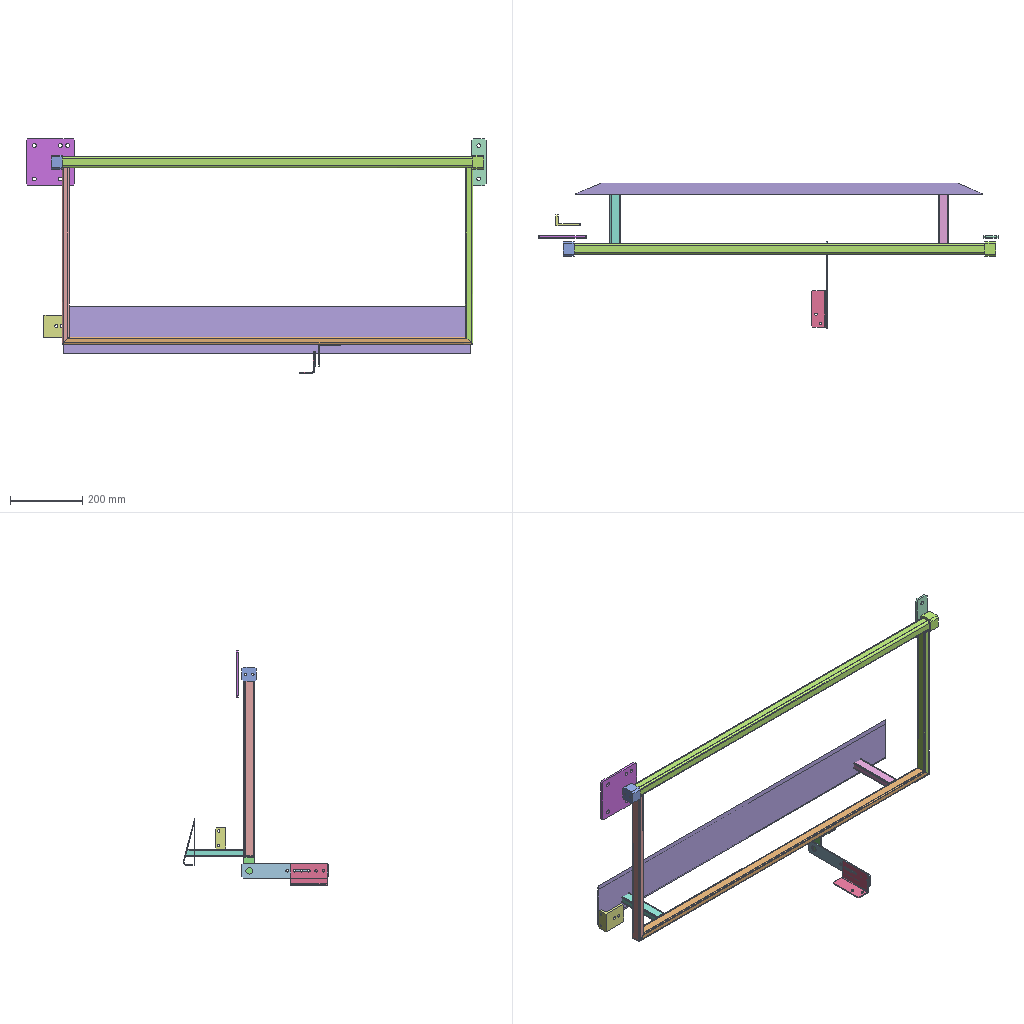Assembly | SolidWorks | 8 different items | 8 placed | box 1271 x 403 x 648 mm
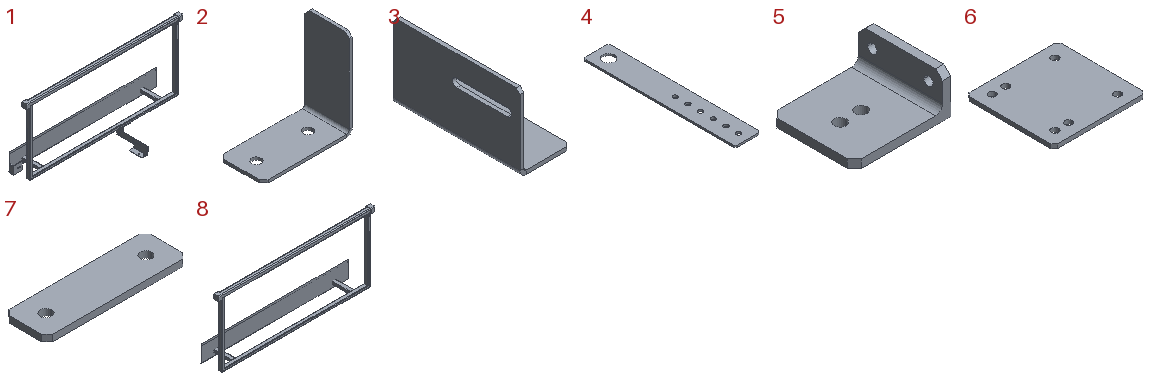Parts list (item | name | quantity | parent item | size | volume | features):
1 | (subassembly) | x1 | - | 1215 x 402.556 x 603 mm | 1534055 mm3 | -
2 | - | x1 | in 1 | 60 x 30 x 60 mm | 6834 mm3 | features Chamfer 1, EdgeFlange 1, FlatPattern 1, ICE 1, SMBaseFlange 1, SheetMetal 1
3 | - | x1 | in 1 | 40 x 100 x 60 mm | 27517 mm3 | features Chamfer 1, EdgeFlange 1, FlatPattern 1, ICE 1, SMBaseFlange 1, SheetMetal 1
4 | - | x1 | in 1 | 40 x 240 x 3 mm | 27247 mm3 | features Extrusion 1
5 | - | x1 | in 1 | 69 x 60 x 30 mm | 32423 mm3 | features ICE 3, Chamfer 1, Extrusion 1, Fillet 1
6 | - | x1 | - | 135 x 130 x 6 mm | 101883 mm3 | features Extrusion 1
7 | - | x1 | - | 130 x 40 x 6 mm | 29861 mm3 | features Extrusion 1
8 | - | x1 | in 1 | 1194 x 202.556 x 548 mm | 1440034 mm3 | features ICE 7, 3DProfileFeature 4, HoleWzd 2, WeldMemberFeat 2, MirrorPattern 1, WeldmentFeature 1
Mates (type | each side: item.copy, entity, surface, feature):
In the top assembly
DistanceDim | 6.1 face plane Boss-Extrude1 | 8.1 face plane Boss-Extrude1
Width | 6.1 face plane Boss-Extrude1 | 6.1 face plane Boss-Extrude1 | 8.1 face plane Boss-Extrude1 | 8.1 face plane Boss-Extrude1
DistanceDim | 7.1 face plane Boss-Extrude1 | 8.1 face plane Mirror1
Width | 7.1 face plane Boss-Extrude1 | 7.1 face plane Boss-Extrude1 | 8.1 face plane Mirror1 | 8.1 face plane Mirror1
In subassembly 1
DistanceDim | 2.1 face plane Edge-Flange1 | 4.1 face plane Boss-Extrude1
Coincident | 2.1 face plane Edge-Flange1 | 4.1 face plane Boss-Extrude1
DistanceDim | 4.1 face plane Boss-Extrude1 | 2.1 face plane Edge-Flange1
Coincident | 3.1 face plane Edge-Flange1 | 4.1 face plane Boss-Extrude1
Concentric | 3.1 face cylinder Cut-Extrude1 | 4.1 face cylinder Boss-Extrude1
Parallel | 3.1 face plane Cut-Extrude1 | 4.1 face plane Boss-Extrude1
Coincident | 8.2 face plane Cold-formed hollow rectangular steel for structures(gb t6728-2002) 30×20×2(2) | 2.1 face plane Base-Flange1
Concentric | 8.2 face cylinder M6 Tapped Hole1 | 2.1 face cylinder Cut-Extrude1 | 2 times
DistanceDim | 5.1 face plane Boss-Extrude1 | 8.2 face plane Cold-formed hollow rectangular steel for structures(gb t6728-2002) 30×20×2(2) | 3 times